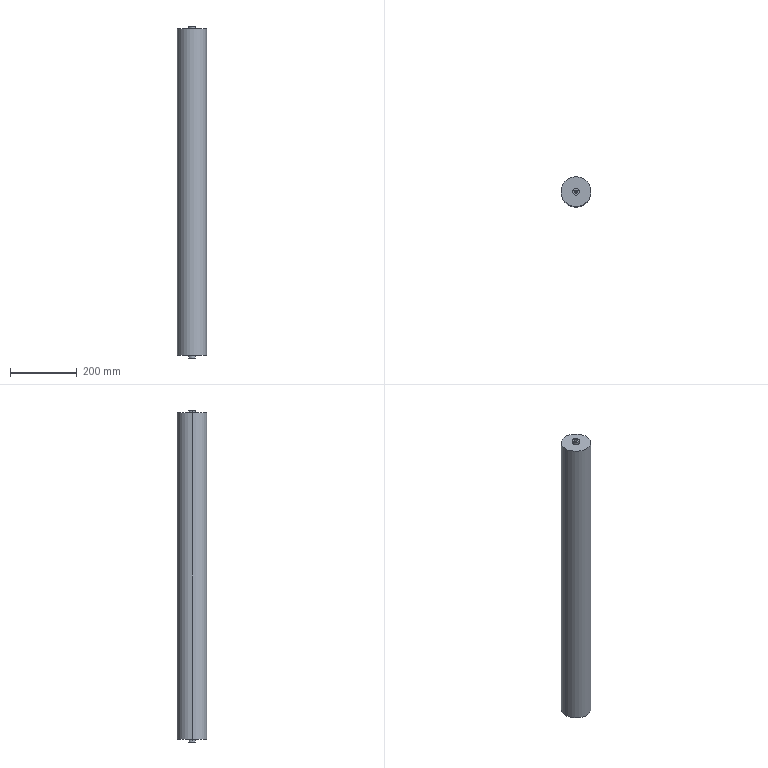Part | SolidWorks | features ICE 3, HoleWzd 2, Extrusion 1 | 1 solid | 18 faces | box 89 x 89 x 992 mm | volume 5903477 mm3 | cylinder 12 | plane 6 | commonest cylinder face diameters 8.5 x4 20 x4 15 x2 89 x2
STEP:
#1=CARTESIAN_POINT('',(-7.5,0.,0.));
#2=VERTEX_POINT('',#1);
#3=CARTESIAN_POINT('',(7.5,0.,0.));
#4=VERTEX_POINT('',#3);
#5=CARTESIAN_POINT('',(0.,0.,0.));
#6=DIRECTION('',(0.,0.,1.));
#7=DIRECTION('',(1.,0.,0.));
#8=AXIS2_PLACEMENT_3D('',#5,#6,#7);
#9=CIRCLE('',#8,7.5);
#10=EDGE_CURVE('',#2,#4,#9,.T.);
#11=ORIENTED_EDGE('',*,*,#10,.F.);
#12=CARTESIAN_POINT('',(-7.5,0.,976.));
#13=VERTEX_POINT('',#12);
#14=CARTESIAN_POINT('',(-7.5,0.,0.));
#15=DIRECTION('',(0.,0.,1.));
#16=VECTOR('',#15,1000.);
#17=LINE('',#14,#16);
#18=EDGE_CURVE('',#2,#13,#17,.T.);
#19=ORIENTED_EDGE('',*,*,#18,.T.);
#20=CARTESIAN_POINT('',(7.5,0.,976.));
#21=VERTEX_POINT('',#20);
#22=CARTESIAN_POINT('',(0.,0.,976.));
#23=DIRECTION('',(0.,0.,1.));
#24=DIRECTION('',(1.,0.,0.));
#25=AXIS2_PLACEMENT_3D('',#22,#23,#24);
#26=CIRCLE('',#25,7.5);
#27=EDGE_CURVE('',#13,#21,#26,.T.);
#28=ORIENTED_EDGE('',*,*,#27,.T.);
#29=CARTESIAN_POINT('',(7.5,0.,0.));
#30=DIRECTION('',(0.,0.,1.));
#31=VECTOR('',#30,1000.);
#32=LINE('',#29,#31);
#33=EDGE_CURVE('',#4,#21,#32,.T.);
#34=ORIENTED_EDGE('',*,*,#33,.F.);
#35=EDGE_LOOP('',(#11,#19,#28,#34));
#36=FACE_OUTER_BOUND('',#35,.T.);
#37=CARTESIAN_POINT('',(0.,0.,0.));
#38=DIRECTION('',(0.,0.,1.));
#39=DIRECTION('',(1.,0.,0.));
#40=AXIS2_PLACEMENT_3D('',#37,#38,#39);
#41=CYLINDRICAL_SURFACE('',#40,7.5);
#42=ADVANCED_FACE('',(#36),#41,.F.);
#43=CARTESIAN_POINT('',(4.25,0.,976.));
#44=VERTEX_POINT('',#43);
#45=CARTESIAN_POINT('',(-4.25,0.,976.));
#46=VERTEX_POINT('',#45);
#47=CARTESIAN_POINT('',(0.,0.,976.));
#48=DIRECTION('',(0.,0.,-1.));
#49=DIRECTION('',(1.,0.,0.));
#50=AXIS2_PLACEMENT_3D('',#47,#48,#49);
#51=CIRCLE('',#50,4.25);
#52=EDGE_CURVE('',#44,#46,#51,.T.);
#53=ORIENTED_EDGE('',*,*,#52,.T.);
#54=CARTESIAN_POINT('',(-4.25,0.,984.));
#55=VERTEX_POINT('',#54);
#56=CARTESIAN_POINT('',(-4.25,0.,984.));
#57=DIRECTION('',(0.,0.,1.));
#58=VECTOR('',#57,1000.);
#59=LINE('',#56,#58);
#60=EDGE_CURVE('',#46,#55,#59,.T.);
#61=ORIENTED_EDGE('',*,*,#60,.T.);
#62=CARTESIAN_POINT('',(4.25,0.,984.));
#63=VERTEX_POINT('',#62);
#64=CARTESIAN_POINT('',(0.,0.,984.));
#65=DIRECTION('',(0.,0.,1.));
#66=DIRECTION('',(1.,0.,0.));
#67=AXIS2_PLACEMENT_3D('',#64,#65,#66);
#68=CIRCLE('',#67,4.25);
#69=EDGE_CURVE('',#55,#63,#68,.T.);
#70=ORIENTED_EDGE('',*,*,#69,.T.);
#71=CARTESIAN_POINT('',(4.25,0.,984.));
#72=DIRECTION('',(0.,0.,1.));
#73=VECTOR('',#72,1000.);
#74=LINE('',#71,#73);
#75=EDGE_CURVE('',#44,#63,#74,.T.);
#76=ORIENTED_EDGE('',*,*,#75,.F.);
#77=EDGE_LOOP('',(#53,#61,#70,#76));
#78=FACE_OUTER_BOUND('',#77,.T.);
#79=CARTESIAN_POINT('',(0.,0.,984.));
#80=DIRECTION('',(0.,0.,1.));
#81=DIRECTION('',(1.,0.,0.));
#82=AXIS2_PLACEMENT_3D('',#79,#80,#81);
#83=CYLINDRICAL_SURFACE('',#82,4.25);
#84=ADVANCED_FACE('',(#78),#83,.F.);
#85=CARTESIAN_POINT('',(-10.,0.,-8.));
#86=VERTEX_POINT('',#85);
#87=CARTESIAN_POINT('',(10.,0.,-8.));
#88=VERTEX_POINT('',#87);
#89=CARTESIAN_POINT('',(0.,0.,-8.));
#90=DIRECTION('',(0.,0.,-1.));
#91=DIRECTION('',(-1.,0.,0.));
#92=AXIS2_PLACEMENT_3D('',#89,#90,#91);
#93=CIRCLE('',#92,10.);
#94=EDGE_CURVE('',#86,#88,#93,.T.);
#95=ORIENTED_EDGE('',*,*,#94,.F.);
#96=CARTESIAN_POINT('',(-10.,0.,0.));
#97=VERTEX_POINT('',#96);
#98=CARTESIAN_POINT('',(-10.,0.,-8.));
#99=DIRECTION('',(0.,0.,1.));
#100=VECTOR('',#99,1000.);
#101=LINE('',#98,#100);
#102=EDGE_CURVE('',#86,#97,#101,.T.);
#103=ORIENTED_EDGE('',*,*,#102,.T.);
#104=CARTESIAN_POINT('',(10.,0.,0.));
#105=VERTEX_POINT('',#104);
#106=CARTESIAN_POINT('',(0.,0.,0.));
#107=DIRECTION('',(0.,0.,-1.));
#108=DIRECTION('',(-1.,0.,0.));
#109=AXIS2_PLACEMENT_3D('',#106,#107,#108);
#110=CIRCLE('',#109,10.);
#111=EDGE_CURVE('',#97,#105,#110,.T.);
#112=ORIENTED_EDGE('',*,*,#111,.T.);
#113=CARTESIAN_POINT('',(10.,0.,-8.));
#114=DIRECTION('',(0.,0.,1.));
#115=VECTOR('',#114,1000.);
#116=LINE('',#113,#115);
#117=EDGE_CURVE('',#88,#105,#116,.T.);
#118=ORIENTED_EDGE('',*,*,#117,.F.);
#119=EDGE_LOOP('',(#95,#103,#112,#118));
#120=FACE_OUTER_BOUND('',#119,.T.);
#121=CARTESIAN_POINT('',(0.,0.,-8.));
#122=DIRECTION('',(0.,0.,1.));
#123=DIRECTION('',(1.,0.,0.));
#124=AXIS2_PLACEMENT_3D('',#121,#122,#123);
#125=CYLINDRICAL_SURFACE('',#124,10.);
#126=ADVANCED_FACE('',(#120),#125,.T.);
#127=CARTESIAN_POINT('',(10.,0.,984.));
#128=VERTEX_POINT('',#127);
#129=CARTESIAN_POINT('',(-10.,0.,984.));
#130=VERTEX_POINT('',#129);
#131=CARTESIAN_POINT('',(0.,0.,984.));
#132=DIRECTION('',(0.,0.,1.));
#133=DIRECTION('',(1.,0.,0.));
#134=AXIS2_PLACEMENT_3D('',#131,#132,#133);
#135=CIRCLE('',#134,10.);
#136=EDGE_CURVE('',#128,#130,#135,.T.);
#137=ORIENTED_EDGE('',*,*,#136,.F.);
#138=CARTESIAN_POINT('',(10.,0.,976.));
#139=VERTEX_POINT('',#138);
#140=CARTESIAN_POINT('',(10.,0.,984.));
#141=DIRECTION('',(0.,0.,-1.));
#142=VECTOR('',#141,1000.);
#143=LINE('',#140,#142);
#144=EDGE_CURVE('',#128,#139,#143,.T.);
#145=ORIENTED_EDGE('',*,*,#144,.T.);
#146=CARTESIAN_POINT('',(-10.,0.,976.));
#147=VERTEX_POINT('',#146);
#148=CARTESIAN_POINT('',(0.,0.,976.));
#149=DIRECTION('',(0.,0.,1.));
#150=DIRECTION('',(1.,0.,0.));
#151=AXIS2_PLACEMENT_3D('',#148,#149,#150);
#152=CIRCLE('',#151,10.);
#153=EDGE_CURVE('',#139,#147,#152,.T.);
#154=ORIENTED_EDGE('',*,*,#153,.T.);
#155=CARTESIAN_POINT('',(-10.,0.,984.));
#156=DIRECTION('',(0.,0.,-1.));
#157=VECTOR('',#156,1000.);
#158=LINE('',#155,#157);
#159=EDGE_CURVE('',#130,#147,#158,.T.);
#160=ORIENTED_EDGE('',*,*,#159,.F.);
#161=EDGE_LOOP('',(#137,#145,#154,#160));
#162=FACE_OUTER_BOUND('',#161,.T.);
#163=CARTESIAN_POINT('',(0.,0.,984.));
#164=DIRECTION('',(0.,0.,-1.));
#165=DIRECTION('',(-1.,0.,0.));
#166=AXIS2_PLACEMENT_3D('',#163,#164,#165);
#167=CYLINDRICAL_SURFACE('',#166,10.);
#168=ADVANCED_FACE('',(#162),#167,.T.);
#169=CARTESIAN_POINT('',(44.5,0.,976.));
#170=VERTEX_POINT('',#169);
#171=CARTESIAN_POINT('',(-44.5,0.,976.));
#172=VERTEX_POINT('',#171);
#173=CARTESIAN_POINT('',(0.,0.,976.));
#174=DIRECTION('',(0.,0.,1.));
#175=DIRECTION('',(1.,0.,0.));
#176=AXIS2_PLACEMENT_3D('',#173,#174,#175);
#177=CIRCLE('',#176,44.5);
#178=EDGE_CURVE('',#170,#172,#177,.T.);
#179=ORIENTED_EDGE('',*,*,#178,.F.);
#180=CARTESIAN_POINT('',(44.5,0.,0.));
#181=VERTEX_POINT('',#180);
#182=CARTESIAN_POINT('',(44.5,0.,976.));
#183=DIRECTION('',(0.,0.,-1.));
#184=VECTOR('',#183,1000.);
#185=LINE('',#182,#184);
#186=EDGE_CURVE('',#170,#181,#185,.T.);
#187=ORIENTED_EDGE('',*,*,#186,.T.);
#188=CARTESIAN_POINT('',(-44.5,0.,0.));
#189=VERTEX_POINT('',#188);
#190=CARTESIAN_POINT('',(0.,0.,0.));
#191=DIRECTION('',(0.,0.,1.));
#192=DIRECTION('',(1.,0.,0.));
#193=AXIS2_PLACEMENT_3D('',#190,#191,#192);
#194=CIRCLE('',#193,44.5);
#195=EDGE_CURVE('',#181,#189,#194,.T.);
#196=ORIENTED_EDGE('',*,*,#195,.T.);
#197=CARTESIAN_POINT('',(-44.5,0.,976.));
#198=DIRECTION('',(0.,0.,-1.));
#199=VECTOR('',#198,1000.);
#200=LINE('',#197,#199);
#201=EDGE_CURVE('',#172,#189,#200,.T.);
#202=ORIENTED_EDGE('',*,*,#201,.F.);
#203=EDGE_LOOP('',(#179,#187,#196,#202));
#204=FACE_OUTER_BOUND('',#203,.T.);
#205=CARTESIAN_POINT('',(0.,0.,976.));
#206=DIRECTION('',(0.,0.,-1.));
#207=DIRECTION('',(-1.,0.,0.));
#208=AXIS2_PLACEMENT_3D('',#205,#206,#207);
#209=CYLINDRICAL_SURFACE('',#208,44.5);
#210=ADVANCED_FACE('',(#204),#209,.T.);
#211=CARTESIAN_POINT('',(4.25,0.,0.));
#212=VERTEX_POINT('',#211);
#213=CARTESIAN_POINT('',(-4.25,0.,0.));
#214=VERTEX_POINT('',#213);
#215=CARTESIAN_POINT('',(0.,0.,0.));
#216=DIRECTION('',(0.,0.,-1.));
#217=DIRECTION('',(1.,0.,0.));
#218=AXIS2_PLACEMENT_3D('',#215,#216,#217);
#219=CIRCLE('',#218,4.25);
#220=EDGE_CURVE('',#212,#214,#219,.T.);
#221=ORIENTED_EDGE('',*,*,#220,.F.);
#222=CARTESIAN_POINT('',(4.25,0.,-8.));
#223=VERTEX_POINT('',#222);
#224=CARTESIAN_POINT('',(4.25,0.,-8.));
#225=DIRECTION('',(0.,0.,-1.));
#226=VECTOR('',#225,1000.);
#227=LINE('',#224,#226);
#228=EDGE_CURVE('',#212,#223,#227,.T.);
#229=ORIENTED_EDGE('',*,*,#228,.T.);
#230=CARTESIAN_POINT('',(-4.25,0.,-8.));
#231=VERTEX_POINT('',#230);
#232=CARTESIAN_POINT('',(0.,0.,-8.));
#233=DIRECTION('',(0.,0.,-1.));
#234=DIRECTION('',(-1.,0.,0.));
#235=AXIS2_PLACEMENT_3D('',#232,#233,#234);
#236=CIRCLE('',#235,4.25);
#237=EDGE_CURVE('',#223,#231,#236,.T.);
#238=ORIENTED_EDGE('',*,*,#237,.T.);
#239=CARTESIAN_POINT('',(-4.25,0.,-8.));
#240=DIRECTION('',(0.,0.,-1.));
#241=VECTOR('',#240,1000.);
#242=LINE('',#239,#241);
#243=EDGE_CURVE('',#214,#231,#242,.T.);
#244=ORIENTED_EDGE('',*,*,#243,.F.);
#245=EDGE_LOOP('',(#221,#229,#238,#244));
#246=FACE_OUTER_BOUND('',#245,.T.);
#247=CARTESIAN_POINT('',(0.,0.,-8.));
#248=DIRECTION('',(0.,0.,-1.));
#249=DIRECTION('',(-1.,0.,0.));
#250=AXIS2_PLACEMENT_3D('',#247,#248,#249);
#251=CYLINDRICAL_SURFACE('',#250,4.25);
#252=ADVANCED_FACE('',(#246),#251,.F.);
#253=ORIENTED_EDGE('',*,*,#228,.F.);
#254=CARTESIAN_POINT('',(0.,0.,0.));
#255=DIRECTION('',(0.,0.,-1.));
#256=DIRECTION('',(1.,0.,0.));
#257=AXIS2_PLACEMENT_3D('',#254,#255,#256);
#258=CIRCLE('',#257,4.25);
#259=EDGE_CURVE('',#214,#212,#258,.T.);
#260=ORIENTED_EDGE('',*,*,#259,.F.);
#261=ORIENTED_EDGE('',*,*,#243,.T.);
#262=CARTESIAN_POINT('',(0.,0.,-8.));
#263=DIRECTION('',(0.,0.,-1.));
#264=DIRECTION('',(-1.,0.,0.));
#265=AXIS2_PLACEMENT_3D('',#262,#263,#264);
#266=CIRCLE('',#265,4.25);
#267=EDGE_CURVE('',#231,#223,#266,.T.);
#268=ORIENTED_EDGE('',*,*,#267,.T.);
#269=EDGE_LOOP('',(#253,#260,#261,#268));
#270=FACE_OUTER_BOUND('',#269,.T.);
#271=CARTESIAN_POINT('',(0.,0.,-8.));
#272=DIRECTION('',(0.,0.,-1.));
#273=DIRECTION('',(-1.,0.,0.));
#274=AXIS2_PLACEMENT_3D('',#271,#272,#273);
#275=CYLINDRICAL_SURFACE('',#274,4.25);
#276=ADVANCED_FACE('',(#270),#275,.F.);
#277=ORIENTED_EDGE('',*,*,#186,.F.);
#278=CARTESIAN_POINT('',(0.,0.,976.));
#279=DIRECTION('',(0.,0.,1.));
#280=DIRECTION('',(1.,0.,0.));
#281=AXIS2_PLACEMENT_3D('',#278,#279,#280);
#282=CIRCLE('',#281,44.5);
#283=EDGE_CURVE('',#172,#170,#282,.T.);
#284=ORIENTED_EDGE('',*,*,#283,.F.);
#285=ORIENTED_EDGE('',*,*,#201,.T.);
#286=CARTESIAN_POINT('',(0.,0.,0.));
#287=DIRECTION('',(0.,0.,1.));
#288=DIRECTION('',(1.,0.,0.));
#289=AXIS2_PLACEMENT_3D('',#286,#287,#288);
#290=CIRCLE('',#289,44.5);
#291=EDGE_CURVE('',#189,#181,#290,.T.);
#292=ORIENTED_EDGE('',*,*,#291,.T.);
#293=EDGE_LOOP('',(#277,#284,#285,#292));
#294=FACE_OUTER_BOUND('',#293,.T.);
#295=CARTESIAN_POINT('',(0.,0.,976.));
#296=DIRECTION('',(0.,0.,-1.));
#297=DIRECTION('',(-1.,0.,0.));
#298=AXIS2_PLACEMENT_3D('',#295,#296,#297);
#299=CYLINDRICAL_SURFACE('',#298,44.5);
#300=ADVANCED_FACE('',(#294),#299,.T.);
#301=CARTESIAN_POINT('',(0.,0.,976.));
#302=DIRECTION('',(0.,0.,1.));
#303=DIRECTION('',(1.,0.,0.));
#304=AXIS2_PLACEMENT_3D('',#301,#302,#303);
#305=CIRCLE('',#304,10.);
#306=EDGE_CURVE('',#147,#139,#305,.T.);
#307=ORIENTED_EDGE('',*,*,#306,.F.);
#308=ORIENTED_EDGE('',*,*,#153,.F.);
#309=EDGE_LOOP('',(#307,#308));
#310=FACE_BOUND('',#309,.T.);
#311=ORIENTED_EDGE('',*,*,#283,.T.);
#312=ORIENTED_EDGE('',*,*,#178,.T.);
#313=EDGE_LOOP('',(#311,#312));
#314=FACE_OUTER_BOUND('',#313,.T.);
#315=CARTESIAN_POINT('',(0.,0.,976.));
#316=DIRECTION('',(0.,0.,1.));
#317=DIRECTION('',(1.,0.,0.));
#318=AXIS2_PLACEMENT_3D('',#315,#316,#317);
#319=PLANE('',#318);
#320=ADVANCED_FACE('',(#310,#314),#319,.T.);
#321=CARTESIAN_POINT('',(0.,0.,0.));
#322=DIRECTION('',(0.,0.,-1.));
#323=DIRECTION('',(-1.,0.,0.));
#324=AXIS2_PLACEMENT_3D('',#321,#322,#323);
#325=CIRCLE('',#324,10.);
#326=EDGE_CURVE('',#105,#97,#325,.T.);
#327=ORIENTED_EDGE('',*,*,#326,.F.);
#328=ORIENTED_EDGE('',*,*,#111,.F.);
#329=EDGE_LOOP('',(#327,#328));
#330=FACE_BOUND('',#329,.T.);
#331=ORIENTED_EDGE('',*,*,#291,.F.);
#332=ORIENTED_EDGE('',*,*,#195,.F.);
#333=EDGE_LOOP('',(#331,#332));
#334=FACE_OUTER_BOUND('',#333,.T.);
#335=CARTESIAN_POINT('',(0.,0.,0.));
#336=DIRECTION('',(0.,0.,1.));
#337=DIRECTION('',(1.,0.,0.));
#338=AXIS2_PLACEMENT_3D('',#335,#336,#337);
#339=PLANE('',#338);
#340=ADVANCED_FACE('',(#330,#334),#339,.F.);
#341=ORIENTED_EDGE('',*,*,#144,.F.);
#342=CARTESIAN_POINT('',(0.,0.,984.));
#343=DIRECTION('',(0.,0.,1.));
#344=DIRECTION('',(1.,0.,0.));
#345=AXIS2_PLACEMENT_3D('',#342,#343,#344);
#346=CIRCLE('',#345,10.);
#347=EDGE_CURVE('',#130,#128,#346,.T.);
#348=ORIENTED_EDGE('',*,*,#347,.F.);
#349=ORIENTED_EDGE('',*,*,#159,.T.);
#350=ORIENTED_EDGE('',*,*,#306,.T.);
#351=EDGE_LOOP('',(#341,#348,#349,#350));
#352=FACE_OUTER_BOUND('',#351,.T.);
#353=CARTESIAN_POINT('',(0.,0.,984.));
#354=DIRECTION('',(0.,0.,-1.));
#355=DIRECTION('',(-1.,0.,0.));
#356=AXIS2_PLACEMENT_3D('',#353,#354,#355);
#357=CYLINDRICAL_SURFACE('',#356,10.);
#358=ADVANCED_FACE('',(#352),#357,.T.);
#359=CARTESIAN_POINT('',(0.,0.,984.));
#360=DIRECTION('',(0.,0.,1.));
#361=DIRECTION('',(1.,0.,0.));
#362=AXIS2_PLACEMENT_3D('',#359,#360,#361);
#363=CIRCLE('',#362,4.25);
#364=EDGE_CURVE('',#63,#55,#363,.T.);
#365=ORIENTED_EDGE('',*,*,#364,.F.);
#366=ORIENTED_EDGE('',*,*,#69,.F.);
#367=EDGE_LOOP('',(#365,#366));
#368=FACE_BOUND('',#367,.T.);
#369=ORIENTED_EDGE('',*,*,#347,.T.);
#370=ORIENTED_EDGE('',*,*,#136,.T.);
#371=EDGE_LOOP('',(#369,#370));
#372=FACE_OUTER_BOUND('',#371,.T.);
#373=CARTESIAN_POINT('',(0.,0.,984.));
#374=DIRECTION('',(0.,0.,1.));
#375=DIRECTION('',(1.,0.,0.));
#376=AXIS2_PLACEMENT_3D('',#373,#374,#375);
#377=PLANE('',#376);
#378=ADVANCED_FACE('',(#368,#372),#377,.T.);
#379=ORIENTED_EDGE('',*,*,#102,.F.);
#380=CARTESIAN_POINT('',(0.,0.,-8.));
#381=DIRECTION('',(0.,0.,-1.));
#382=DIRECTION('',(-1.,0.,0.));
#383=AXIS2_PLACEMENT_3D('',#380,#381,#382);
#384=CIRCLE('',#383,10.);
#385=EDGE_CURVE('',#88,#86,#384,.T.);
#386=ORIENTED_EDGE('',*,*,#385,.F.);
#387=ORIENTED_EDGE('',*,*,#117,.T.);
#388=ORIENTED_EDGE('',*,*,#326,.T.);
#389=EDGE_LOOP('',(#379,#386,#387,#388));
#390=FACE_OUTER_BOUND('',#389,.T.);
#391=CARTESIAN_POINT('',(0.,0.,-8.));
#392=DIRECTION('',(0.,0.,1.));
#393=DIRECTION('',(1.,0.,0.));
#394=AXIS2_PLACEMENT_3D('',#391,#392,#393);
#395=CYLINDRICAL_SURFACE('',#394,10.);
#396=ADVANCED_FACE('',(#390),#395,.T.);
#397=ORIENTED_EDGE('',*,*,#267,.F.);
#398=ORIENTED_EDGE('',*,*,#237,.F.);
#399=EDGE_LOOP('',(#397,#398));
#400=FACE_BOUND('',#399,.T.);
#401=ORIENTED_EDGE('',*,*,#385,.T.);
#402=ORIENTED_EDGE('',*,*,#94,.T.);
#403=EDGE_LOOP('',(#401,#402));
#404=FACE_OUTER_BOUND('',#403,.T.);
#405=CARTESIAN_POINT('',(0.,0.,-8.));
#406=DIRECTION('',(0.,0.,-1.));
#407=DIRECTION('',(-1.,0.,0.));
#408=AXIS2_PLACEMENT_3D('',#405,#406,#407);
#409=PLANE('',#408);
#410=ADVANCED_FACE('',(#400,#404),#409,.T.);
#411=ORIENTED_EDGE('',*,*,#60,.F.);
#412=CARTESIAN_POINT('',(0.,0.,976.));
#413=DIRECTION('',(0.,0.,-1.));
#414=DIRECTION('',(1.,0.,0.));
#415=AXIS2_PLACEMENT_3D('',#412,#413,#414);
#416=CIRCLE('',#415,4.25);
#417=EDGE_CURVE('',#46,#44,#416,.T.);
#418=ORIENTED_EDGE('',*,*,#417,.T.);
#419=ORIENTED_EDGE('',*,*,#75,.T.);
#420=ORIENTED_EDGE('',*,*,#364,.T.);
#421=EDGE_LOOP('',(#411,#418,#419,#420));
#422=FACE_OUTER_BOUND('',#421,.T.);
#423=CARTESIAN_POINT('',(0.,0.,984.));
#424=DIRECTION('',(0.,0.,1.));
#425=DIRECTION('',(1.,0.,0.));
#426=AXIS2_PLACEMENT_3D('',#423,#424,#425);
#427=CYLINDRICAL_SURFACE('',#426,4.25);
#428=ADVANCED_FACE('',(#422),#427,.F.);
#429=CARTESIAN_POINT('',(0.,0.,0.));
#430=DIRECTION('',(0.,0.,1.));
#431=DIRECTION('',(1.,0.,0.));
#432=AXIS2_PLACEMENT_3D('',#429,#430,#431);
#433=CIRCLE('',#432,7.5);
#434=EDGE_CURVE('',#4,#2,#433,.T.);
#435=ORIENTED_EDGE('',*,*,#434,.T.);
#436=ORIENTED_EDGE('',*,*,#10,.T.);
#437=EDGE_LOOP('',(#435,#436));
#438=FACE_OUTER_BOUND('',#437,.T.);
#439=ORIENTED_EDGE('',*,*,#259,.T.);
#440=ORIENTED_EDGE('',*,*,#220,.T.);
#441=EDGE_LOOP('',(#439,#440));
#442=FACE_BOUND('',#441,.T.);
#443=CARTESIAN_POINT('',(0.,0.,0.));
#444=DIRECTION('',(0.,0.,1.));
#445=DIRECTION('',(1.,0.,0.));
#446=AXIS2_PLACEMENT_3D('',#443,#444,#445);
#447=PLANE('',#446);
#448=ADVANCED_FACE('',(#438,#442),#447,.T.);
#449=CARTESIAN_POINT('',(0.,0.,976.));
#450=DIRECTION('',(0.,0.,1.));
#451=DIRECTION('',(1.,0.,0.));
#452=AXIS2_PLACEMENT_3D('',#449,#450,#451);
#453=CIRCLE('',#452,7.5);
#454=EDGE_CURVE('',#21,#13,#453,.T.);
#455=ORIENTED_EDGE('',*,*,#454,.F.);
#456=ORIENTED_EDGE('',*,*,#27,.F.);
#457=EDGE_LOOP('',(#455,#456));
#458=FACE_OUTER_BOUND('',#457,.T.);
#459=ORIENTED_EDGE('',*,*,#52,.F.);
#460=ORIENTED_EDGE('',*,*,#417,.F.);
#461=EDGE_LOOP('',(#459,#460));
#462=FACE_BOUND('',#461,.T.);
#463=CARTESIAN_POINT('',(0.,0.,976.));
#464=DIRECTION('',(0.,0.,1.));
#465=DIRECTION('',(1.,0.,0.));
#466=AXIS2_PLACEMENT_3D('',#463,#464,#465);
#467=PLANE('',#466);
#468=ADVANCED_FACE('',(#458,#462),#467,.F.);
#469=ORIENTED_EDGE('',*,*,#18,.F.);
#470=ORIENTED_EDGE('',*,*,#434,.F.);
#471=ORIENTED_EDGE('',*,*,#33,.T.);
#472=ORIENTED_EDGE('',*,*,#454,.T.);
#473=EDGE_LOOP('',(#469,#470,#471,#472));
#474=FACE_OUTER_BOUND('',#473,.T.);
#475=CARTESIAN_POINT('',(0.,0.,0.));
#476=DIRECTION('',(0.,0.,1.));
#477=DIRECTION('',(1.,0.,0.));
#478=AXIS2_PLACEMENT_3D('',#475,#476,#477);
#479=CYLINDRICAL_SURFACE('',#478,7.5);
#480=ADVANCED_FACE('',(#474),#479,.F.);
#481=CLOSED_SHELL('',(#42,#84,#126,#168,#210,#252,#276,#300,#320,#340,#358,#378,#396,#410,#428,#448,#468,#480));
#482=MANIFOLD_SOLID_BREP('',#481);
#483=CARTESIAN_POINT('',(0.,0.,0.));
#484=DIRECTION('',(0.,0.,1.));
#485=DIRECTION('',(1.,0.,0.));
#486=AXIS2_PLACEMENT_3D('',#483,#484,#485);
#487=(LENGTH_UNIT()NAMED_UNIT(*)SI_UNIT(.MILLI.,.METRE.));
#488=UNCERTAINTY_MEASURE_WITH_UNIT(LENGTH_MEASURE(0.00001),#487,'','');
#489=(NAMED_UNIT(*)PLANE_ANGLE_UNIT()SI_UNIT($,.RADIAN.));
#490=(NAMED_UNIT(*)SI_UNIT($,.STERADIAN.)SOLID_ANGLE_UNIT());
#491=(GEOMETRIC_REPRESENTATION_CONTEXT(3)GLOBAL_UNCERTAINTY_ASSIGNED_CONTEXT((#488))GLOBAL_UNIT_ASSIGNED_CONTEXT((#487,#489,#490))REPRESENTATION_CONTEXT('',''));
#492=ADVANCED_BREP_SHAPE_REPRESENTATION('',(#482,#486),#491);